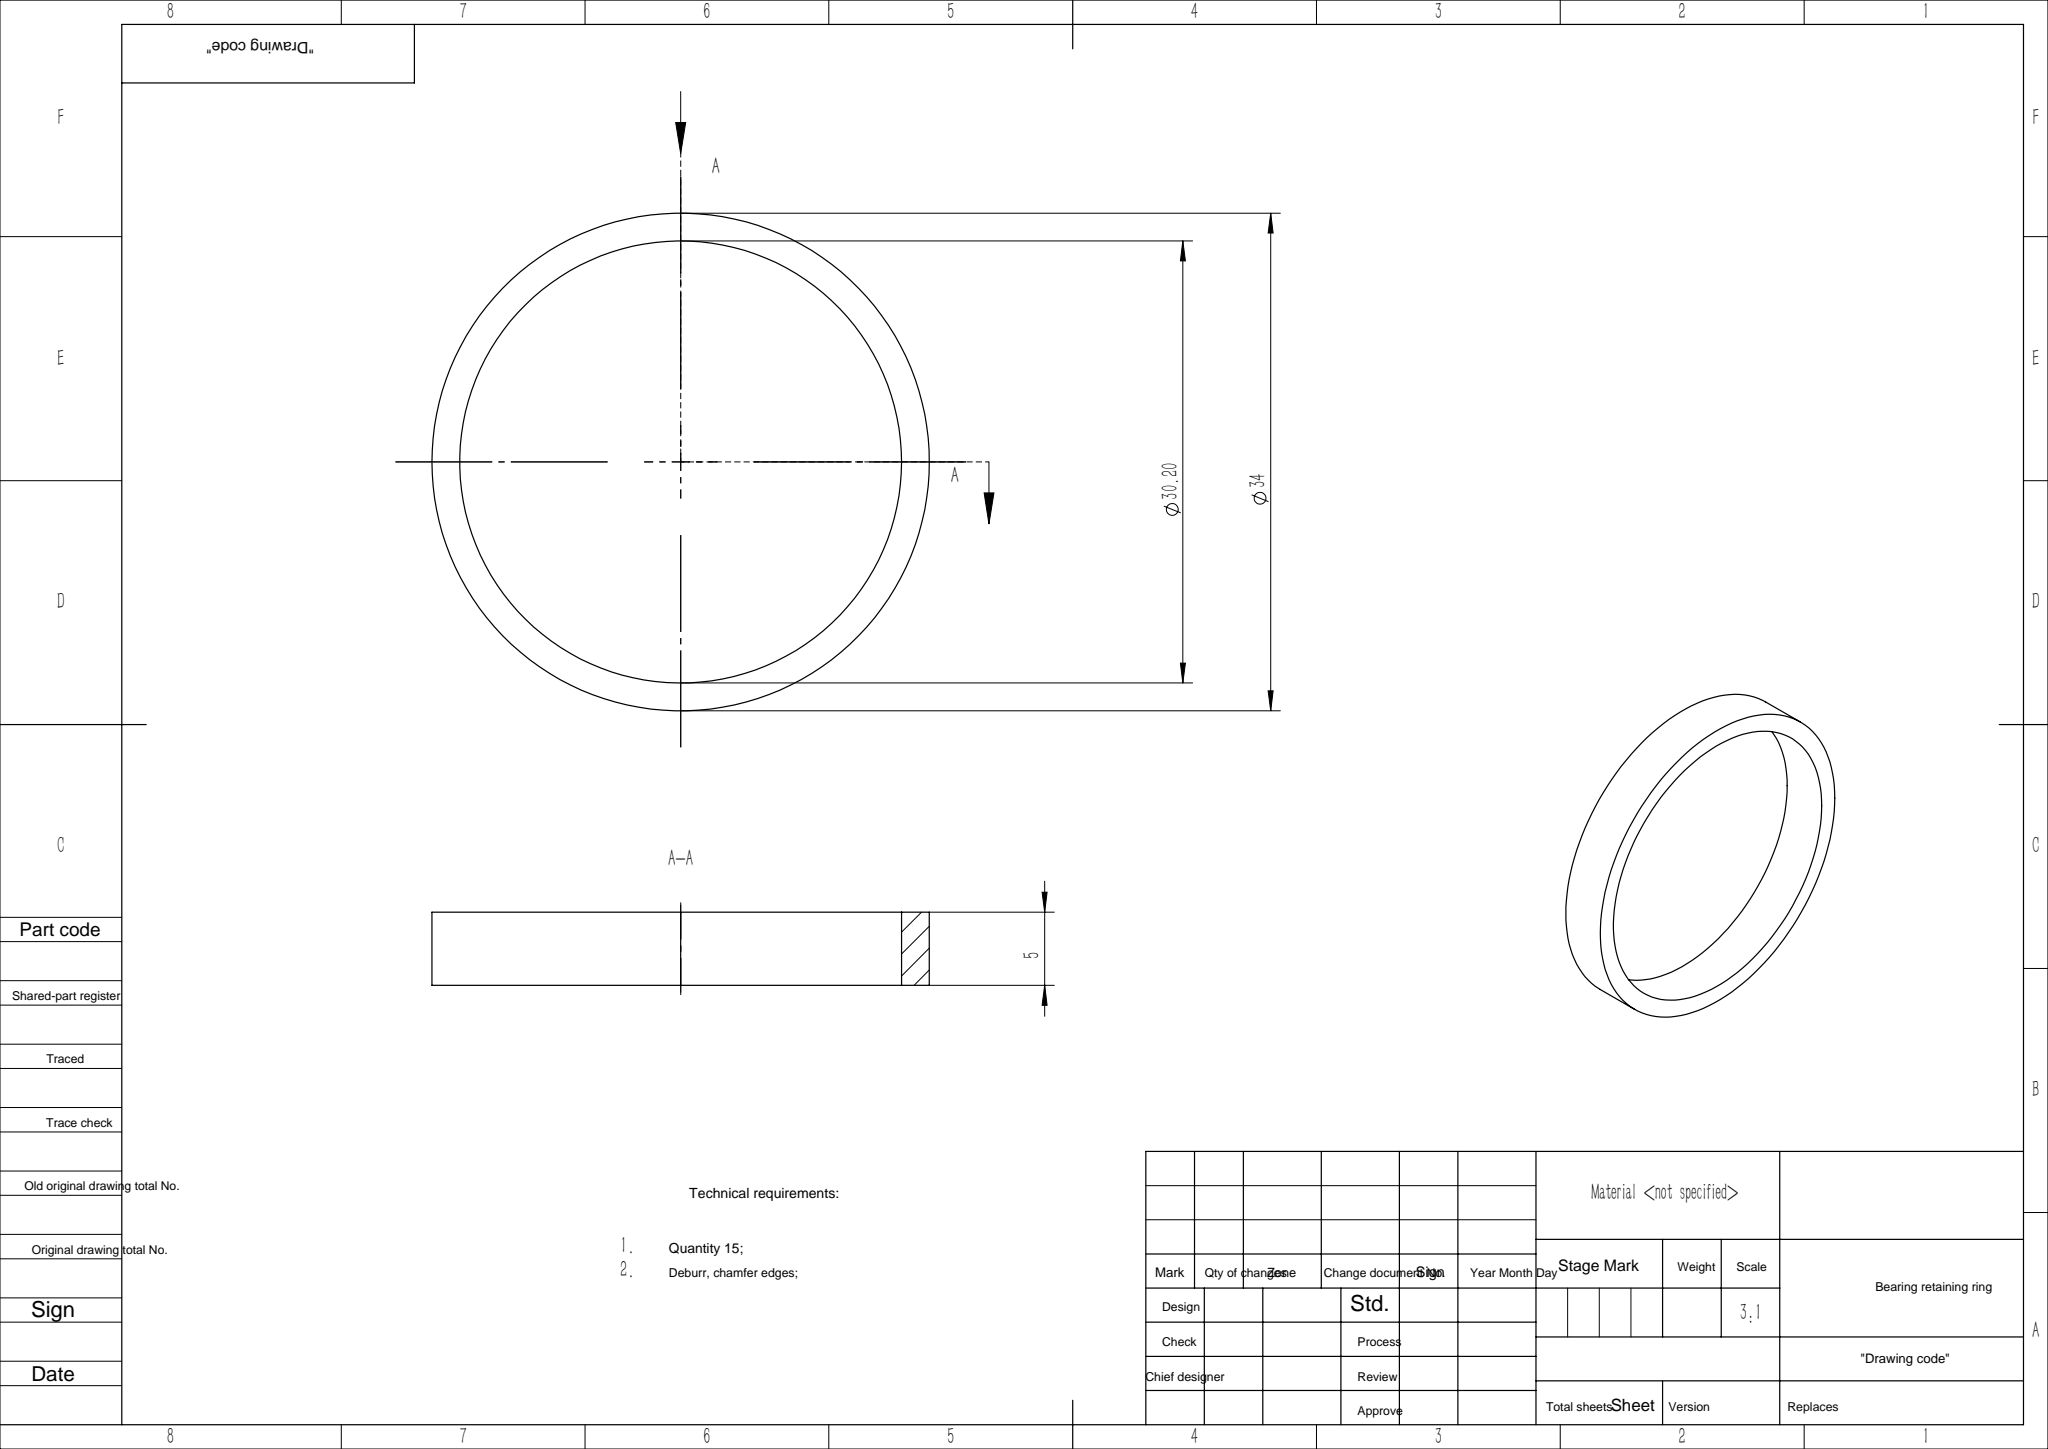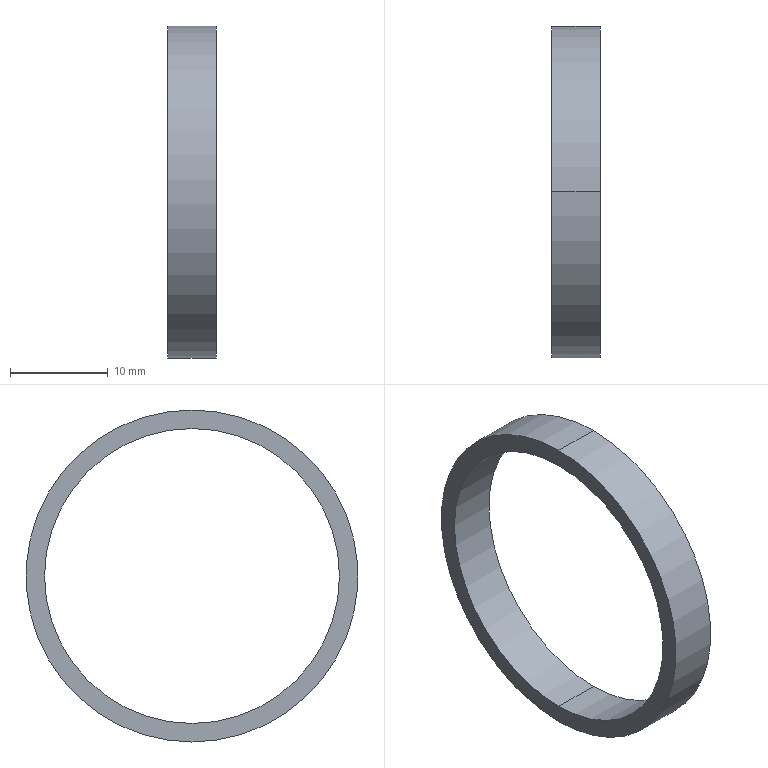Part | SolidWorks | features Extrusion 1 | 1 solid | 6 faces | box 5 x 34 x 34 mm | volume 958.029 mm3 | cylinder 4 | plane 2 | commonest cylinder face diameters 30.2 x2 34 x2
STEP:
#1=CARTESIAN_POINT('',(5.,0.,15.1));
#2=VERTEX_POINT('',#1);
#3=CARTESIAN_POINT('',(5.,0.,-15.1));
#4=VERTEX_POINT('',#3);
#5=CARTESIAN_POINT('',(5.,0.,0.));
#6=DIRECTION('',(1.,0.,0.));
#7=DIRECTION('',(0.,0.,-1.));
#8=AXIS2_PLACEMENT_3D('',#5,#6,#7);
#9=CIRCLE('',#8,15.1);
#10=EDGE_CURVE('',#2,#4,#9,.T.);
#11=ORIENTED_EDGE('',*,*,#10,.T.);
#12=CARTESIAN_POINT('',(0.,0.,-15.1));
#13=VERTEX_POINT('',#12);
#14=CARTESIAN_POINT('',(5.,0.,-15.1));
#15=DIRECTION('',(-1.,0.,0.));
#16=VECTOR('',#15,1000.);
#17=LINE('',#14,#16);
#18=EDGE_CURVE('',#4,#13,#17,.T.);
#19=ORIENTED_EDGE('',*,*,#18,.T.);
#20=CARTESIAN_POINT('',(0.,0.,15.1));
#21=VERTEX_POINT('',#20);
#22=CARTESIAN_POINT('',(0.,0.,0.));
#23=DIRECTION('',(1.,0.,0.));
#24=DIRECTION('',(0.,0.,-1.));
#25=AXIS2_PLACEMENT_3D('',#22,#23,#24);
#26=CIRCLE('',#25,15.1);
#27=EDGE_CURVE('',#21,#13,#26,.T.);
#28=ORIENTED_EDGE('',*,*,#27,.F.);
#29=CARTESIAN_POINT('',(5.,0.,15.1));
#30=DIRECTION('',(-1.,0.,0.));
#31=VECTOR('',#30,1000.);
#32=LINE('',#29,#31);
#33=EDGE_CURVE('',#2,#21,#32,.T.);
#34=ORIENTED_EDGE('',*,*,#33,.F.);
#35=EDGE_LOOP('',(#11,#19,#28,#34));
#36=FACE_OUTER_BOUND('',#35,.T.);
#37=CARTESIAN_POINT('',(5.,0.,0.));
#38=DIRECTION('',(-1.,0.,0.));
#39=DIRECTION('',(0.,0.,1.));
#40=AXIS2_PLACEMENT_3D('',#37,#38,#39);
#41=CYLINDRICAL_SURFACE('',#40,15.1);
#42=ADVANCED_FACE('',(#36),#41,.F.);
#43=CARTESIAN_POINT('',(5.,0.,-17.));
#44=VERTEX_POINT('',#43);
#45=CARTESIAN_POINT('',(5.,0.,17.));
#46=VERTEX_POINT('',#45);
#47=CARTESIAN_POINT('',(5.,0.,0.));
#48=DIRECTION('',(1.,0.,0.));
#49=DIRECTION('',(0.,0.,-1.));
#50=AXIS2_PLACEMENT_3D('',#47,#48,#49);
#51=CIRCLE('',#50,17.);
#52=EDGE_CURVE('',#44,#46,#51,.T.);
#53=ORIENTED_EDGE('',*,*,#52,.F.);
#54=CARTESIAN_POINT('',(0.,0.,-17.));
#55=VERTEX_POINT('',#54);
#56=CARTESIAN_POINT('',(5.,0.,-17.));
#57=DIRECTION('',(-1.,0.,0.));
#58=VECTOR('',#57,1000.);
#59=LINE('',#56,#58);
#60=EDGE_CURVE('',#44,#55,#59,.T.);
#61=ORIENTED_EDGE('',*,*,#60,.T.);
#62=CARTESIAN_POINT('',(0.,0.,17.));
#63=VERTEX_POINT('',#62);
#64=CARTESIAN_POINT('',(0.,0.,0.));
#65=DIRECTION('',(1.,0.,0.));
#66=DIRECTION('',(0.,0.,-1.));
#67=AXIS2_PLACEMENT_3D('',#64,#65,#66);
#68=CIRCLE('',#67,17.);
#69=EDGE_CURVE('',#55,#63,#68,.T.);
#70=ORIENTED_EDGE('',*,*,#69,.T.);
#71=CARTESIAN_POINT('',(5.,0.,17.));
#72=DIRECTION('',(-1.,0.,0.));
#73=VECTOR('',#72,1000.);
#74=LINE('',#71,#73);
#75=EDGE_CURVE('',#46,#63,#74,.T.);
#76=ORIENTED_EDGE('',*,*,#75,.F.);
#77=EDGE_LOOP('',(#53,#61,#70,#76));
#78=FACE_OUTER_BOUND('',#77,.T.);
#79=CARTESIAN_POINT('',(5.,0.,0.));
#80=DIRECTION('',(-1.,0.,0.));
#81=DIRECTION('',(0.,0.,1.));
#82=AXIS2_PLACEMENT_3D('',#79,#80,#81);
#83=CYLINDRICAL_SURFACE('',#82,17.);
#84=ADVANCED_FACE('',(#78),#83,.T.);
#85=CARTESIAN_POINT('',(5.,0.,0.));
#86=DIRECTION('',(1.,0.,0.));
#87=DIRECTION('',(0.,0.,-1.));
#88=AXIS2_PLACEMENT_3D('',#85,#86,#87);
#89=CIRCLE('',#88,17.);
#90=EDGE_CURVE('',#46,#44,#89,.T.);
#91=ORIENTED_EDGE('',*,*,#90,.T.);
#92=ORIENTED_EDGE('',*,*,#52,.T.);
#93=EDGE_LOOP('',(#91,#92));
#94=FACE_OUTER_BOUND('',#93,.T.);
#95=ORIENTED_EDGE('',*,*,#10,.F.);
#96=CARTESIAN_POINT('',(5.,0.,0.));
#97=DIRECTION('',(1.,0.,0.));
#98=DIRECTION('',(0.,0.,-1.));
#99=AXIS2_PLACEMENT_3D('',#96,#97,#98);
#100=CIRCLE('',#99,15.1);
#101=EDGE_CURVE('',#4,#2,#100,.T.);
#102=ORIENTED_EDGE('',*,*,#101,.F.);
#103=EDGE_LOOP('',(#95,#102));
#104=FACE_BOUND('',#103,.T.);
#105=CARTESIAN_POINT('',(5.,0.,0.));
#106=DIRECTION('',(1.,0.,0.));
#107=DIRECTION('',(0.,0.,-1.));
#108=AXIS2_PLACEMENT_3D('',#105,#106,#107);
#109=PLANE('',#108);
#110=ADVANCED_FACE('',(#94,#104),#109,.T.);
#111=CARTESIAN_POINT('',(0.,0.,0.));
#112=DIRECTION('',(1.,0.,0.));
#113=DIRECTION('',(0.,0.,-1.));
#114=AXIS2_PLACEMENT_3D('',#111,#112,#113);
#115=CIRCLE('',#114,17.);
#116=EDGE_CURVE('',#63,#55,#115,.T.);
#117=ORIENTED_EDGE('',*,*,#116,.F.);
#118=ORIENTED_EDGE('',*,*,#69,.F.);
#119=EDGE_LOOP('',(#117,#118));
#120=FACE_OUTER_BOUND('',#119,.T.);
#121=ORIENTED_EDGE('',*,*,#27,.T.);
#122=CARTESIAN_POINT('',(0.,0.,0.));
#123=DIRECTION('',(1.,0.,0.));
#124=DIRECTION('',(0.,0.,-1.));
#125=AXIS2_PLACEMENT_3D('',#122,#123,#124);
#126=CIRCLE('',#125,15.1);
#127=EDGE_CURVE('',#13,#21,#126,.T.);
#128=ORIENTED_EDGE('',*,*,#127,.T.);
#129=EDGE_LOOP('',(#121,#128));
#130=FACE_BOUND('',#129,.T.);
#131=CARTESIAN_POINT('',(0.,0.,0.));
#132=DIRECTION('',(1.,0.,0.));
#133=DIRECTION('',(0.,0.,-1.));
#134=AXIS2_PLACEMENT_3D('',#131,#132,#133);
#135=PLANE('',#134);
#136=ADVANCED_FACE('',(#120,#130),#135,.F.);
#137=ORIENTED_EDGE('',*,*,#60,.F.);
#138=ORIENTED_EDGE('',*,*,#90,.F.);
#139=ORIENTED_EDGE('',*,*,#75,.T.);
#140=ORIENTED_EDGE('',*,*,#116,.T.);
#141=EDGE_LOOP('',(#137,#138,#139,#140));
#142=FACE_OUTER_BOUND('',#141,.T.);
#143=CARTESIAN_POINT('',(5.,0.,0.));
#144=DIRECTION('',(-1.,0.,0.));
#145=DIRECTION('',(0.,0.,1.));
#146=AXIS2_PLACEMENT_3D('',#143,#144,#145);
#147=CYLINDRICAL_SURFACE('',#146,17.);
#148=ADVANCED_FACE('',(#142),#147,.T.);
#149=ORIENTED_EDGE('',*,*,#18,.F.);
#150=ORIENTED_EDGE('',*,*,#101,.T.);
#151=ORIENTED_EDGE('',*,*,#33,.T.);
#152=ORIENTED_EDGE('',*,*,#127,.F.);
#153=EDGE_LOOP('',(#149,#150,#151,#152));
#154=FACE_OUTER_BOUND('',#153,.T.);
#155=CARTESIAN_POINT('',(5.,0.,0.));
#156=DIRECTION('',(-1.,0.,0.));
#157=DIRECTION('',(0.,0.,1.));
#158=AXIS2_PLACEMENT_3D('',#155,#156,#157);
#159=CYLINDRICAL_SURFACE('',#158,15.1);
#160=ADVANCED_FACE('',(#154),#159,.F.);
#161=CLOSED_SHELL('',(#42,#84,#110,#136,#148,#160));
#162=MANIFOLD_SOLID_BREP('',#161);
#163=CARTESIAN_POINT('',(0.,0.,0.));
#164=DIRECTION('',(0.,0.,1.));
#165=DIRECTION('',(1.,0.,0.));
#166=AXIS2_PLACEMENT_3D('',#163,#164,#165);
#167=(LENGTH_UNIT()NAMED_UNIT(*)SI_UNIT(.MILLI.,.METRE.));
#168=UNCERTAINTY_MEASURE_WITH_UNIT(LENGTH_MEASURE(0.00001),#167,'','');
#169=(NAMED_UNIT(*)PLANE_ANGLE_UNIT()SI_UNIT($,.RADIAN.));
#170=(NAMED_UNIT(*)SI_UNIT($,.STERADIAN.)SOLID_ANGLE_UNIT());
#171=(GEOMETRIC_REPRESENTATION_CONTEXT(3)GLOBAL_UNCERTAINTY_ASSIGNED_CONTEXT((#168))GLOBAL_UNIT_ASSIGNED_CONTEXT((#167,#169,#170))REPRESENTATION_CONTEXT('',''));
#172=ADVANCED_BREP_SHAPE_REPRESENTATION('',(#162,#166),#171);